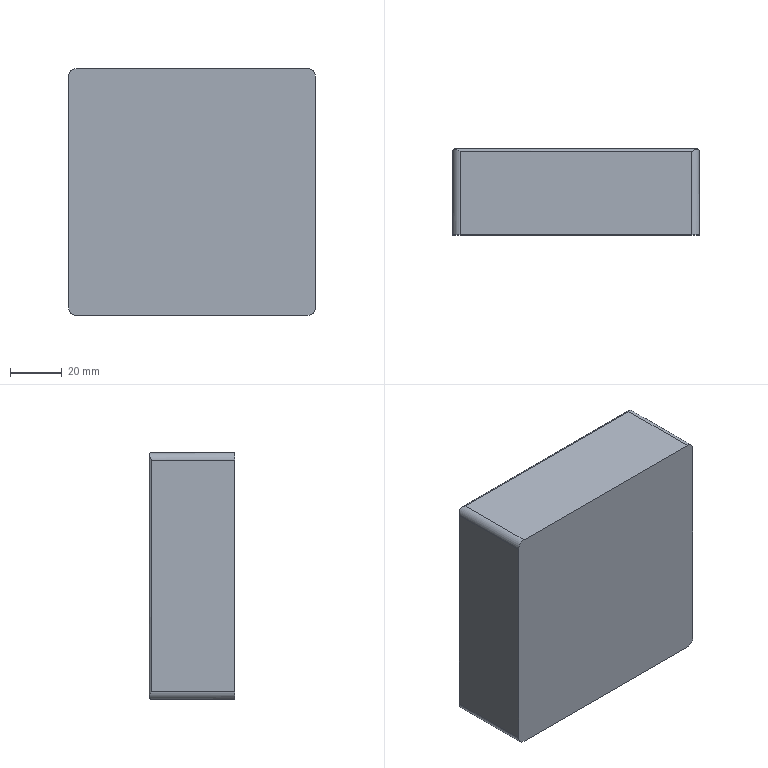Part | SolidWorks | features BaseBody 1 | 1 solid | 20 faces | box 95 x 33 x 95 mm | volume 297490 mm3 | cylinder 9 | plane 6 | cone 5 | commonest cylinder face diameters 2 x5 6 x4
STEP:
#1=CARTESIAN_POINT('',(155.5,-10.5,-46.5));
#2=VERTEX_POINT('',#1);
#3=CARTESIAN_POINT('',(154.5,-10.5,-47.5));
#4=VERTEX_POINT('',#3);
#5=CARTESIAN_POINT('',(154.5,-10.5,-47.5));
#6=DIRECTION('',(-0.7071,0.,-0.7071));
#7=VECTOR('',#6,1000.);
#8=LINE('',#5,#7);
#9=EDGE_CURVE('',#2,#4,#8,.T.);
#10=ORIENTED_EDGE('',*,*,#9,.F.);
#11=CARTESIAN_POINT('',(156.5,-10.5,-47.5));
#12=VERTEX_POINT('',#11);
#13=CARTESIAN_POINT('',(156.5,-10.5,-47.5));
#14=DIRECTION('',(0.7071,0.,-0.7071));
#15=VECTOR('',#14,1000.);
#16=LINE('',#13,#15);
#17=EDGE_CURVE('',#2,#12,#16,.T.);
#18=ORIENTED_EDGE('',*,*,#17,.T.);
#19=CARTESIAN_POINT('',(155.5,-10.5,-47.5));
#20=DIRECTION('',(0.,0.,1.));
#21=DIRECTION('',(-1.,0.,0.));
#22=AXIS2_PLACEMENT_3D('',#19,#20,#21);
#23=CIRCLE('',#22,1.);
#24=EDGE_CURVE('',#4,#12,#23,.T.);
#25=ORIENTED_EDGE('',*,*,#24,.F.);
#26=EDGE_LOOP('',(#10,#18,#25));
#27=FACE_OUTER_BOUND('',#26,.T.);
#28=CARTESIAN_POINT('',(155.5,-10.5,-47.5));
#29=DIRECTION('',(0.,0.,-1.));
#30=DIRECTION('',(-1.,0.,0.));
#31=AXIS2_PLACEMENT_3D('',#28,#29,#30);
#32=CONICAL_SURFACE('',#31,1.,0.7854);
#33=ADVANCED_FACE('',(#27),#32,.F.);
#34=CARTESIAN_POINT('',(182.5,-10.5,-46.5));
#35=VERTEX_POINT('',#34);
#36=CARTESIAN_POINT('',(181.5,-10.5,-47.5));
#37=VERTEX_POINT('',#36);
#38=CARTESIAN_POINT('',(181.5,-10.5,-47.5));
#39=DIRECTION('',(-0.7071,0.,-0.7071));
#40=VECTOR('',#39,1000.);
#41=LINE('',#38,#40);
#42=EDGE_CURVE('',#35,#37,#41,.T.);
#43=ORIENTED_EDGE('',*,*,#42,.F.);
#44=CARTESIAN_POINT('',(183.5,-10.5,-47.5));
#45=VERTEX_POINT('',#44);
#46=CARTESIAN_POINT('',(183.5,-10.5,-47.5));
#47=DIRECTION('',(0.7071,0.,-0.7071));
#48=VECTOR('',#47,1000.);
#49=LINE('',#46,#48);
#50=EDGE_CURVE('',#35,#45,#49,.T.);
#51=ORIENTED_EDGE('',*,*,#50,.T.);
#52=CARTESIAN_POINT('',(182.5,-10.5,-47.5));
#53=DIRECTION('',(0.,0.,1.));
#54=DIRECTION('',(-1.,0.,0.));
#55=AXIS2_PLACEMENT_3D('',#52,#53,#54);
#56=CIRCLE('',#55,1.);
#57=EDGE_CURVE('',#37,#45,#56,.T.);
#58=ORIENTED_EDGE('',*,*,#57,.F.);
#59=EDGE_LOOP('',(#43,#51,#58));
#60=FACE_OUTER_BOUND('',#59,.T.);
#61=CARTESIAN_POINT('',(182.5,-10.5,-47.5));
#62=DIRECTION('',(0.,0.,-1.));
#63=DIRECTION('',(-1.,0.,0.));
#64=AXIS2_PLACEMENT_3D('',#61,#62,#63);
#65=CONICAL_SURFACE('',#64,1.,0.7854);
#66=ADVANCED_FACE('',(#60),#65,.F.);
#67=CARTESIAN_POINT('',(218.,-26.,44.5));
#68=VERTEX_POINT('',#67);
#69=CARTESIAN_POINT('',(215.,-26.,47.5));
#70=VERTEX_POINT('',#69);
#71=CARTESIAN_POINT('',(215.,-26.,44.5));
#72=DIRECTION('',(0.,-1.,0.));
#73=DIRECTION('',(0.,0.,-1.));
#74=AXIS2_PLACEMENT_3D('',#71,#72,#73);
#75=CIRCLE('',#74,3.);
#76=EDGE_CURVE('',#68,#70,#75,.T.);
#77=ORIENTED_EDGE('',*,*,#76,.T.);
#78=CARTESIAN_POINT('',(126.,-26.,47.5));
#79=VERTEX_POINT('',#78);
#80=CARTESIAN_POINT('',(170.5,-26.,47.5));
#81=DIRECTION('',(-1.,0.,0.));
#82=VECTOR('',#81,1000.);
#83=LINE('',#80,#82);
#84=EDGE_CURVE('',#70,#79,#83,.T.);
#85=ORIENTED_EDGE('',*,*,#84,.T.);
#86=CARTESIAN_POINT('',(123.,-26.,44.5));
#87=VERTEX_POINT('',#86);
#88=CARTESIAN_POINT('',(126.,-26.,44.5));
#89=DIRECTION('',(0.,-1.,0.));
#90=DIRECTION('',(0.,0.,-1.));
#91=AXIS2_PLACEMENT_3D('',#88,#89,#90);
#92=CIRCLE('',#91,3.);
#93=EDGE_CURVE('',#79,#87,#92,.T.);
#94=ORIENTED_EDGE('',*,*,#93,.T.);
#95=CARTESIAN_POINT('',(123.,-26.,-44.5));
#96=VERTEX_POINT('',#95);
#97=CARTESIAN_POINT('',(123.,-26.,0.));
#98=DIRECTION('',(0.,0.,-1.));
#99=VECTOR('',#98,1000.);
#100=LINE('',#97,#99);
#101=EDGE_CURVE('',#87,#96,#100,.T.);
#102=ORIENTED_EDGE('',*,*,#101,.T.);
#103=CARTESIAN_POINT('',(126.,-26.,-47.5));
#104=VERTEX_POINT('',#103);
#105=CARTESIAN_POINT('',(126.,-26.,-44.5));
#106=DIRECTION('',(0.,-1.,0.));
#107=DIRECTION('',(0.,0.,-1.));
#108=AXIS2_PLACEMENT_3D('',#105,#106,#107);
#109=CIRCLE('',#108,3.);
#110=EDGE_CURVE('',#96,#104,#109,.T.);
#111=ORIENTED_EDGE('',*,*,#110,.T.);
#112=CARTESIAN_POINT('',(215.,-26.,-47.5));
#113=VERTEX_POINT('',#112);
#114=CARTESIAN_POINT('',(170.5,-26.,-47.5));
#115=DIRECTION('',(1.,0.,0.));
#116=VECTOR('',#115,1000.);
#117=LINE('',#114,#116);
#118=EDGE_CURVE('',#104,#113,#117,.T.);
#119=ORIENTED_EDGE('',*,*,#118,.T.);
#120=CARTESIAN_POINT('',(218.,-26.,-44.5));
#121=VERTEX_POINT('',#120);
#122=CARTESIAN_POINT('',(215.,-26.,-44.5));
#123=DIRECTION('',(0.,-1.,0.));
#124=DIRECTION('',(0.,0.,-1.));
#125=AXIS2_PLACEMENT_3D('',#122,#123,#124);
#126=CIRCLE('',#125,3.);
#127=EDGE_CURVE('',#113,#121,#126,.T.);
#128=ORIENTED_EDGE('',*,*,#127,.T.);
#129=CARTESIAN_POINT('',(218.,-26.,0.));
#130=DIRECTION('',(0.,0.,1.));
#131=VECTOR('',#130,1000.);
#132=LINE('',#129,#131);
#133=EDGE_CURVE('',#121,#68,#132,.T.);
#134=ORIENTED_EDGE('',*,*,#133,.T.);
#135=EDGE_LOOP('',(#77,#85,#94,#102,#111,#119,#128,#134));
#136=FACE_OUTER_BOUND('',#135,.T.);
#137=CARTESIAN_POINT('',(170.5,-26.,0.));
#138=DIRECTION('',(0.,-1.,0.));
#139=DIRECTION('',(0.,0.,-1.));
#140=AXIS2_PLACEMENT_3D('',#137,#138,#139);
#141=PLANE('',#140);
#142=ADVANCED_FACE('',(#136),#141,.T.);
#143=CARTESIAN_POINT('',(215.,6.,47.5));
#144=VERTEX_POINT('',#143);
#145=CARTESIAN_POINT('',(215.,7.,47.5));
#146=DIRECTION('',(0.,1.,0.));
#147=VECTOR('',#146,1000.);
#148=LINE('',#145,#147);
#149=EDGE_CURVE('',#70,#144,#148,.T.);
#150=ORIENTED_EDGE('',*,*,#149,.T.);
#151=CARTESIAN_POINT('',(126.,6.,47.5));
#152=VERTEX_POINT('',#151);
#153=CARTESIAN_POINT('',(126.,6.,47.5));
#154=DIRECTION('',(-1.,0.,0.));
#155=VECTOR('',#154,1000.);
#156=LINE('',#153,#155);
#157=EDGE_CURVE('',#144,#152,#156,.T.);
#158=ORIENTED_EDGE('',*,*,#157,.T.);
#159=CARTESIAN_POINT('',(126.,7.,47.5));
#160=DIRECTION('',(0.,-1.,0.));
#161=VECTOR('',#160,1000.);
#162=LINE('',#159,#161);
#163=EDGE_CURVE('',#152,#79,#162,.T.);
#164=ORIENTED_EDGE('',*,*,#163,.T.);
#165=ORIENTED_EDGE('',*,*,#84,.F.);
#166=EDGE_LOOP('',(#150,#158,#164,#165));
#167=FACE_OUTER_BOUND('',#166,.T.);
#168=CARTESIAN_POINT('',(126.,7.,47.5));
#169=DIRECTION('',(0.,0.,1.));
#170=DIRECTION('',(1.,0.,0.));
#171=AXIS2_PLACEMENT_3D('',#168,#169,#170);
#172=PLANE('',#171);
#173=ADVANCED_FACE('',(#167),#172,.T.);
#174=CARTESIAN_POINT('',(218.,6.,44.5));
#175=VERTEX_POINT('',#174);
#176=CARTESIAN_POINT('',(218.,7.,44.5));
#177=DIRECTION('',(0.,1.,0.));
#178=VECTOR('',#177,1000.);
#179=LINE('',#176,#178);
#180=EDGE_CURVE('',#68,#175,#179,.T.);
#181=ORIENTED_EDGE('',*,*,#180,.T.);
#182=CARTESIAN_POINT('',(217.121,6.993,46.621));
#183=VERTEX_POINT('',#182);
#184=CARTESIAN_POINT('',(218.,6.,44.5));
#185=CARTESIAN_POINT('',(218.,6.053,44.592));
#186=CARTESIAN_POINT('',(217.996,6.108,44.686));
#187=CARTESIAN_POINT('',(217.978,6.214,44.871));
#188=CARTESIAN_POINT('',(217.965,6.266,44.963));
#189=CARTESIAN_POINT('',(217.914,6.421,45.238));
#190=CARTESIAN_POINT('',(217.862,6.52,45.42));
#191=CARTESIAN_POINT('',(217.718,6.705,45.784));
#192=CARTESIAN_POINT('',(217.628,6.789,45.961));
#193=CARTESIAN_POINT('',(217.406,6.923,46.303));
#194=CARTESIAN_POINT('',(217.273,6.974,46.469));
#195=CARTESIAN_POINT('',(217.121,6.993,46.621));
#196=B_SPLINE_CURVE_WITH_KNOTS('',3,(#184,#185,#186,#187,#188,#189,#190,#191,#192,#193,#194,#195),.UNSPECIFIED.,.F.,.F.,(4,2,2,2,2,4),(-0.00001095,0.0003086,0.0006282,0.001267,0.001907,0.002546),.UNSPECIFIED.);
#197=EDGE_CURVE('',#175,#183,#196,.T.);
#198=ORIENTED_EDGE('',*,*,#197,.T.);
#199=CARTESIAN_POINT('',(217.121,6.993,46.621));
#200=CARTESIAN_POINT('',(216.968,6.974,46.774));
#201=CARTESIAN_POINT('',(216.806,6.924,46.904));
#202=CARTESIAN_POINT('',(216.461,6.789,47.128));
#203=CARTESIAN_POINT('',(216.285,6.706,47.218));
#204=CARTESIAN_POINT('',(215.746,6.432,47.431));
#205=CARTESIAN_POINT('',(215.371,6.214,47.5));
#206=CARTESIAN_POINT('',(215.,6.,47.5));
#207=B_SPLINE_CURVE_WITH_KNOTS('',3,(#199,#200,#201,#202,#203,#204,#205,#206),.UNSPECIFIED.,.F.,.F.,(4,2,2,4),(0.,0.0006423,0.001285,0.002569),.UNSPECIFIED.);
#208=EDGE_CURVE('',#183,#144,#207,.T.);
#209=ORIENTED_EDGE('',*,*,#208,.T.);
#210=ORIENTED_EDGE('',*,*,#149,.F.);
#211=ORIENTED_EDGE('',*,*,#76,.F.);
#212=EDGE_LOOP('',(#181,#198,#209,#210,#211));
#213=FACE_OUTER_BOUND('',#212,.T.);
#214=CARTESIAN_POINT('',(215.,7.,44.5));
#215=DIRECTION('',(0.,-1.,0.));
#216=DIRECTION('',(0.,0.,-1.));
#217=AXIS2_PLACEMENT_3D('',#214,#215,#216);
#218=CYLINDRICAL_SURFACE('',#217,3.);
#219=ADVANCED_FACE('',(#213),#218,.T.);
#220=CARTESIAN_POINT('',(218.,6.,-44.5));
#221=VERTEX_POINT('',#220);
#222=CARTESIAN_POINT('',(218.,7.,-44.5));
#223=DIRECTION('',(0.,1.,0.));
#224=VECTOR('',#223,1000.);
#225=LINE('',#222,#224);
#226=EDGE_CURVE('',#121,#221,#225,.T.);
#227=ORIENTED_EDGE('',*,*,#226,.T.);
#228=CARTESIAN_POINT('',(218.,6.,44.5));
#229=DIRECTION('',(0.,0.,1.));
#230=VECTOR('',#229,1000.);
#231=LINE('',#228,#230);
#232=EDGE_CURVE('',#221,#175,#231,.T.);
#233=ORIENTED_EDGE('',*,*,#232,.T.);
#234=ORIENTED_EDGE('',*,*,#180,.F.);
#235=ORIENTED_EDGE('',*,*,#133,.F.);
#236=EDGE_LOOP('',(#227,#233,#234,#235));
#237=FACE_OUTER_BOUND('',#236,.T.);
#238=CARTESIAN_POINT('',(218.,7.,44.5));
#239=DIRECTION('',(1.,0.,0.));
#240=DIRECTION('',(0.,0.,-1.));
#241=AXIS2_PLACEMENT_3D('',#238,#239,#240);
#242=PLANE('',#241);
#243=ADVANCED_FACE('',(#237),#242,.T.);
#244=ORIENTED_EDGE('',*,*,#127,.F.);
#245=CARTESIAN_POINT('',(215.,6.,-47.5));
#246=VERTEX_POINT('',#245);
#247=CARTESIAN_POINT('',(215.,7.,-47.5));
#248=DIRECTION('',(0.,1.,0.));
#249=VECTOR('',#248,1000.);
#250=LINE('',#247,#249);
#251=EDGE_CURVE('',#113,#246,#250,.T.);
#252=ORIENTED_EDGE('',*,*,#251,.T.);
#253=CARTESIAN_POINT('',(217.121,6.993,-46.621));
#254=VERTEX_POINT('',#253);
#255=CARTESIAN_POINT('',(215.,6.,-47.5));
#256=CARTESIAN_POINT('',(215.092,6.053,-47.5));
#257=CARTESIAN_POINT('',(215.186,6.108,-47.496));
#258=CARTESIAN_POINT('',(215.371,6.214,-47.478));
#259=CARTESIAN_POINT('',(215.463,6.266,-47.465));
#260=CARTESIAN_POINT('',(215.738,6.421,-47.414));
#261=CARTESIAN_POINT('',(215.92,6.52,-47.362));
#262=CARTESIAN_POINT('',(216.284,6.705,-47.218));
#263=CARTESIAN_POINT('',(216.461,6.789,-47.128));
#264=CARTESIAN_POINT('',(216.803,6.923,-46.906));
#265=CARTESIAN_POINT('',(216.969,6.974,-46.773));
#266=CARTESIAN_POINT('',(217.121,6.993,-46.621));
#267=B_SPLINE_CURVE_WITH_KNOTS('',3,(#255,#256,#257,#258,#259,#260,#261,#262,#263,#264,#265,#266),.UNSPECIFIED.,.F.,.F.,(4,2,2,2,2,4),(-0.00001095,0.0003086,0.0006282,0.001267,0.001907,0.002546),.UNSPECIFIED.);
#268=EDGE_CURVE('',#246,#254,#267,.T.);
#269=ORIENTED_EDGE('',*,*,#268,.T.);
#270=CARTESIAN_POINT('',(217.121,6.993,-46.621));
#271=CARTESIAN_POINT('',(217.274,6.974,-46.468));
#272=CARTESIAN_POINT('',(217.404,6.924,-46.306));
#273=CARTESIAN_POINT('',(217.628,6.789,-45.961));
#274=CARTESIAN_POINT('',(217.718,6.706,-45.785));
#275=CARTESIAN_POINT('',(217.931,6.432,-45.246));
#276=CARTESIAN_POINT('',(218.,6.214,-44.871));
#277=CARTESIAN_POINT('',(218.,6.,-44.5));
#278=B_SPLINE_CURVE_WITH_KNOTS('',3,(#270,#271,#272,#273,#274,#275,#276,#277),.UNSPECIFIED.,.F.,.F.,(4,2,2,4),(0.,0.0006423,0.001285,0.002569),.UNSPECIFIED.);
#279=EDGE_CURVE('',#254,#221,#278,.T.);
#280=ORIENTED_EDGE('',*,*,#279,.T.);
#281=ORIENTED_EDGE('',*,*,#226,.F.);
#282=EDGE_LOOP('',(#244,#252,#269,#280,#281));
#283=FACE_OUTER_BOUND('',#282,.T.);
#284=CARTESIAN_POINT('',(215.,7.,-44.5));
#285=DIRECTION('',(0.,-1.,0.));
#286=DIRECTION('',(0.,0.,-1.));
#287=AXIS2_PLACEMENT_3D('',#284,#285,#286);
#288=CYLINDRICAL_SURFACE('',#287,3.);
#289=ADVANCED_FACE('',(#283),#288,.T.);
#290=CARTESIAN_POINT('',(126.,6.,-47.5));
#291=VERTEX_POINT('',#290);
#292=CARTESIAN_POINT('',(182.5,6.,-47.5));
#293=VERTEX_POINT('',#292);
#294=CARTESIAN_POINT('',(215.,6.,-47.5));
#295=DIRECTION('',(1.,0.,0.));
#296=VECTOR('',#295,1000.);
#297=LINE('',#294,#296);
#298=EDGE_CURVE('',#291,#293,#297,.T.);
#299=ORIENTED_EDGE('',*,*,#298,.T.);
#300=CARTESIAN_POINT('',(215.,6.,-47.5));
#301=DIRECTION('',(1.,0.,0.));
#302=VECTOR('',#301,1000.);
#303=LINE('',#300,#302);
#304=EDGE_CURVE('',#293,#246,#303,.T.);
#305=ORIENTED_EDGE('',*,*,#304,.T.);
#306=ORIENTED_EDGE('',*,*,#251,.F.);
#307=ORIENTED_EDGE('',*,*,#118,.F.);
#308=CARTESIAN_POINT('',(126.,7.,-47.5));
#309=DIRECTION('',(0.,1.,0.));
#310=VECTOR('',#309,1000.);
#311=LINE('',#308,#310);
#312=EDGE_CURVE('',#104,#291,#311,.T.);
#313=ORIENTED_EDGE('',*,*,#312,.T.);
#314=EDGE_LOOP('',(#299,#305,#306,#307,#313));
#315=FACE_OUTER_BOUND('',#314,.T.);
#316=ORIENTED_EDGE('',*,*,#24,.T.);
#317=CARTESIAN_POINT('',(155.5,-10.5,-47.5));
#318=DIRECTION('',(0.,0.,1.));
#319=DIRECTION('',(-1.,0.,0.));
#320=AXIS2_PLACEMENT_3D('',#317,#318,#319);
#321=CIRCLE('',#320,1.);
#322=EDGE_CURVE('',#12,#4,#321,.T.);
#323=ORIENTED_EDGE('',*,*,#322,.T.);
#324=EDGE_LOOP('',(#316,#323));
#325=FACE_BOUND('',#324,.T.);
#326=ORIENTED_EDGE('',*,*,#57,.T.);
#327=CARTESIAN_POINT('',(182.5,-10.5,-47.5));
#328=DIRECTION('',(0.,0.,1.));
#329=DIRECTION('',(-1.,0.,0.));
#330=AXIS2_PLACEMENT_3D('',#327,#328,#329);
#331=CIRCLE('',#330,1.);
#332=EDGE_CURVE('',#45,#37,#331,.T.);
#333=ORIENTED_EDGE('',*,*,#332,.T.);
#334=EDGE_LOOP('',(#326,#333));
#335=FACE_BOUND('',#334,.T.);
#336=CARTESIAN_POINT('',(215.,7.,-47.5));
#337=DIRECTION('',(0.,0.,-1.));
#338=DIRECTION('',(-1.,0.,0.));
#339=AXIS2_PLACEMENT_3D('',#336,#337,#338);
#340=PLANE('',#339);
#341=ADVANCED_FACE('',(#315,#325,#335),#340,.T.);
#342=CARTESIAN_POINT('',(123.,6.,-44.5));
#343=VERTEX_POINT('',#342);
#344=CARTESIAN_POINT('',(123.,7.,-44.5));
#345=DIRECTION('',(0.,1.,0.));
#346=VECTOR('',#345,1000.);
#347=LINE('',#344,#346);
#348=EDGE_CURVE('',#96,#343,#347,.T.);
#349=ORIENTED_EDGE('',*,*,#348,.T.);
#350=CARTESIAN_POINT('',(123.879,6.993,-46.621));
#351=VERTEX_POINT('',#350);
#352=CARTESIAN_POINT('',(123.,6.,-44.5));
#353=CARTESIAN_POINT('',(123.,6.214,-44.871));
#354=CARTESIAN_POINT('',(123.069,6.432,-45.247));
#355=CARTESIAN_POINT('',(123.282,6.706,-45.785));
#356=CARTESIAN_POINT('',(123.372,6.789,-45.961));
#357=CARTESIAN_POINT('',(123.596,6.924,-46.306));
#358=CARTESIAN_POINT('',(123.726,6.974,-46.468));
#359=CARTESIAN_POINT('',(123.879,6.993,-46.621));
#360=B_SPLINE_CURVE_WITH_KNOTS('',3,(#352,#353,#354,#355,#356,#357,#358,#359),.UNSPECIFIED.,.F.,.F.,(4,2,2,4),(-0.00001095,0.001275,0.001919,0.002562),.UNSPECIFIED.);
#361=EDGE_CURVE('',#343,#351,#360,.T.);
#362=ORIENTED_EDGE('',*,*,#361,.T.);
#363=CARTESIAN_POINT('',(123.879,6.993,-46.621));
#364=CARTESIAN_POINT('',(124.032,6.974,-46.774));
#365=CARTESIAN_POINT('',(124.194,6.924,-46.904));
#366=CARTESIAN_POINT('',(124.539,6.789,-47.128));
#367=CARTESIAN_POINT('',(124.715,6.706,-47.218));
#368=CARTESIAN_POINT('',(125.254,6.432,-47.431));
#369=CARTESIAN_POINT('',(125.629,6.214,-47.5));
#370=CARTESIAN_POINT('',(126.,6.,-47.5));
#371=B_SPLINE_CURVE_WITH_KNOTS('',3,(#363,#364,#365,#366,#367,#368,#369,#370),.UNSPECIFIED.,.F.,.F.,(4,2,2,4),(0.,0.0006423,0.001285,0.002569),.UNSPECIFIED.);
#372=EDGE_CURVE('',#351,#291,#371,.T.);
#373=ORIENTED_EDGE('',*,*,#372,.T.);
#374=ORIENTED_EDGE('',*,*,#312,.F.);
#375=ORIENTED_EDGE('',*,*,#110,.F.);
#376=EDGE_LOOP('',(#349,#362,#373,#374,#375));
#377=FACE_OUTER_BOUND('',#376,.T.);
#378=CARTESIAN_POINT('',(126.,7.,-44.5));
#379=DIRECTION('',(0.,-1.,0.));
#380=DIRECTION('',(0.,0.,-1.));
#381=AXIS2_PLACEMENT_3D('',#378,#379,#380);
#382=CYLINDRICAL_SURFACE('',#381,3.);
#383=ADVANCED_FACE('',(#377),#382,.T.);
#384=CARTESIAN_POINT('',(123.,6.,44.5));
#385=VERTEX_POINT('',#384);
#386=CARTESIAN_POINT('',(123.,7.,44.5));
#387=DIRECTION('',(0.,1.,0.));
#388=VECTOR('',#387,1000.);
#389=LINE('',#386,#388);
#390=EDGE_CURVE('',#87,#385,#389,.T.);
#391=ORIENTED_EDGE('',*,*,#390,.T.);
#392=CARTESIAN_POINT('',(123.,6.,0.));
#393=DIRECTION('',(0.,0.,-1.));
#394=VECTOR('',#393,1000.);
#395=LINE('',#392,#394);
#396=EDGE_CURVE('',#385,#343,#395,.T.);
#397=ORIENTED_EDGE('',*,*,#396,.T.);
#398=ORIENTED_EDGE('',*,*,#348,.F.);
#399=ORIENTED_EDGE('',*,*,#101,.F.);
#400=EDGE_LOOP('',(#391,#397,#398,#399));
#401=FACE_OUTER_BOUND('',#400,.T.);
#402=CARTESIAN_POINT('',(123.,7.,0.));
#403=DIRECTION('',(-1.,0.,0.));
#404=DIRECTION('',(0.,0.,1.));
#405=AXIS2_PLACEMENT_3D('',#402,#403,#404);
#406=PLANE('',#405);
#407=ADVANCED_FACE('',(#401),#406,.T.);
#408=ORIENTED_EDGE('',*,*,#93,.F.);
#409=ORIENTED_EDGE('',*,*,#163,.F.);
#410=CARTESIAN_POINT('',(123.879,6.993,46.621));
#411=VERTEX_POINT('',#410);
#412=CARTESIAN_POINT('',(126.,6.,47.5));
#413=CARTESIAN_POINT('',(125.629,6.214,47.5));
#414=CARTESIAN_POINT('',(125.253,6.432,47.431));
#415=CARTESIAN_POINT('',(124.715,6.706,47.218));
#416=CARTESIAN_POINT('',(124.539,6.789,47.128));
#417=CARTESIAN_POINT('',(124.194,6.924,46.904));
#418=CARTESIAN_POINT('',(124.032,6.974,46.774));
#419=CARTESIAN_POINT('',(123.879,6.993,46.621));
#420=B_SPLINE_CURVE_WITH_KNOTS('',3,(#412,#413,#414,#415,#416,#417,#418,#419),.UNSPECIFIED.,.F.,.F.,(4,2,2,4),(-0.00001095,0.001275,0.001919,0.002562),.UNSPECIFIED.);
#421=EDGE_CURVE('',#152,#411,#420,.T.);
#422=ORIENTED_EDGE('',*,*,#421,.T.);
#423=CARTESIAN_POINT('',(123.879,6.993,46.621));
#424=CARTESIAN_POINT('',(123.726,6.974,46.468));
#425=CARTESIAN_POINT('',(123.596,6.924,46.306));
#426=CARTESIAN_POINT('',(123.372,6.789,45.961));
#427=CARTESIAN_POINT('',(123.282,6.706,45.785));
#428=CARTESIAN_POINT('',(123.069,6.432,45.246));
#429=CARTESIAN_POINT('',(123.,6.214,44.871));
#430=CARTESIAN_POINT('',(123.,6.,44.5));
#431=B_SPLINE_CURVE_WITH_KNOTS('',3,(#423,#424,#425,#426,#427,#428,#429,#430),.UNSPECIFIED.,.F.,.F.,(4,2,2,4),(0.,0.0006423,0.001285,0.002569),.UNSPECIFIED.);
#432=EDGE_CURVE('',#411,#385,#431,.T.);
#433=ORIENTED_EDGE('',*,*,#432,.T.);
#434=ORIENTED_EDGE('',*,*,#390,.F.);
#435=EDGE_LOOP('',(#408,#409,#422,#433,#434));
#436=FACE_OUTER_BOUND('',#435,.T.);
#437=CARTESIAN_POINT('',(126.,7.,44.5));
#438=DIRECTION('',(0.,-1.,0.));
#439=DIRECTION('',(0.,0.,-1.));
#440=AXIS2_PLACEMENT_3D('',#437,#438,#439);
#441=CYLINDRICAL_SURFACE('',#440,3.);
#442=ADVANCED_FACE('',(#436),#441,.T.);
#443=ORIENTED_EDGE('',*,*,#421,.F.);
#444=ORIENTED_EDGE('',*,*,#157,.F.);
#445=ORIENTED_EDGE('',*,*,#208,.F.);
#446=CARTESIAN_POINT('',(217.,7.,46.5));
#447=VERTEX_POINT('',#446);
#448=CARTESIAN_POINT('',(217.121,6.993,46.621));
#449=CARTESIAN_POINT('',(217.081,6.998,46.581));
#450=CARTESIAN_POINT('',(217.041,7.,46.541));
#451=CARTESIAN_POINT('',(217.,7.,46.5));
#452=(BOUNDED_CURVE()B_SPLINE_CURVE(3,(#448,#449,#450,#451),.UNSPECIFIED.,.F.,.F.)B_SPLINE_CURVE_WITH_KNOTS((4,4),(4.591,4.712),.UNSPECIFIED.)CURVE()GEOMETRIC_REPRESENTATION_ITEM()RATIONAL_B_SPLINE_CURVE((1.,0.9988,0.9988,1.))REPRESENTATION_ITEM(''));
#453=EDGE_CURVE('',#183,#447,#452,.T.);
#454=ORIENTED_EDGE('',*,*,#453,.T.);
#455=CARTESIAN_POINT('',(124.,7.,46.5));
#456=VERTEX_POINT('',#455);
#457=CARTESIAN_POINT('',(218.,7.,46.5));
#458=DIRECTION('',(-1.,0.,0.));
#459=VECTOR('',#458,1000.);
#460=LINE('',#457,#459);
#461=EDGE_CURVE('',#447,#456,#460,.T.);
#462=ORIENTED_EDGE('',*,*,#461,.T.);
#463=CARTESIAN_POINT('',(124.,7.,46.5));
#464=CARTESIAN_POINT('',(123.959,7.,46.541));
#465=CARTESIAN_POINT('',(123.919,6.998,46.581));
#466=CARTESIAN_POINT('',(123.879,6.993,46.621));
#467=(BOUNDED_CURVE()B_SPLINE_CURVE(3,(#463,#464,#465,#466),.UNSPECIFIED.,.F.,.T.)B_SPLINE_CURVE_WITH_KNOTS((4,4),(4.712,4.834),.UNSPECIFIED.)CURVE()GEOMETRIC_REPRESENTATION_ITEM()RATIONAL_B_SPLINE_CURVE((1.,0.9988,0.9988,1.))REPRESENTATION_ITEM(''));
#468=EDGE_CURVE('',#456,#411,#467,.T.);
#469=ORIENTED_EDGE('',*,*,#468,.T.);
#470=EDGE_LOOP('',(#443,#444,#445,#454,#462,#469));
#471=FACE_OUTER_BOUND('',#470,.T.);
#472=CARTESIAN_POINT('',(218.,6.,46.5));
#473=DIRECTION('',(-1.,0.,0.));
#474=DIRECTION('',(0.,0.,1.));
#475=AXIS2_PLACEMENT_3D('',#472,#473,#474);
#476=CYLINDRICAL_SURFACE('',#475,1.);
#477=ADVANCED_FACE('',(#471),#476,.T.);
#478=ORIENTED_EDGE('',*,*,#232,.F.);
#479=ORIENTED_EDGE('',*,*,#279,.F.);
#480=CARTESIAN_POINT('',(217.,7.,-46.5));
#481=VERTEX_POINT('',#480);
#482=CARTESIAN_POINT('',(217.121,6.993,-46.621));
#483=CARTESIAN_POINT('',(217.081,6.998,-46.581));
#484=CARTESIAN_POINT('',(217.041,7.,-46.541));
#485=CARTESIAN_POINT('',(217.,7.,-46.5));
#486=(BOUNDED_CURVE()B_SPLINE_CURVE(3,(#482,#483,#484,#485),.UNSPECIFIED.,.F.,.F.)B_SPLINE_CURVE_WITH_KNOTS((4,4),(1.449,1.571),.UNSPECIFIED.)CURVE()GEOMETRIC_REPRESENTATION_ITEM()RATIONAL_B_SPLINE_CURVE((1.,0.9988,0.9988,1.))REPRESENTATION_ITEM(''));
#487=EDGE_CURVE('',#254,#481,#486,.T.);
#488=ORIENTED_EDGE('',*,*,#487,.T.);
#489=CARTESIAN_POINT('',(217.,7.,47.5));
#490=DIRECTION('',(0.,0.,1.));
#491=VECTOR('',#490,1000.);
#492=LINE('',#489,#491);
#493=EDGE_CURVE('',#481,#447,#492,.T.);
#494=ORIENTED_EDGE('',*,*,#493,.T.);
#495=ORIENTED_EDGE('',*,*,#453,.F.);
#496=ORIENTED_EDGE('',*,*,#197,.F.);
#497=EDGE_LOOP('',(#478,#479,#488,#494,#495,#496));
#498=FACE_OUTER_BOUND('',#497,.T.);
#499=CARTESIAN_POINT('',(217.,6.,47.5));
#500=DIRECTION('',(0.,0.,-1.));
#501=DIRECTION('',(-1.,0.,0.));
#502=AXIS2_PLACEMENT_3D('',#499,#500,#501);
#503=CYLINDRICAL_SURFACE('',#502,1.);
#504=ADVANCED_FACE('',(#498),#503,.T.);
#505=ORIENTED_EDGE('',*,*,#268,.F.);
#506=ORIENTED_EDGE('',*,*,#304,.F.);
#507=CARTESIAN_POINT('',(182.5,7.,-46.5));
#508=VERTEX_POINT('',#507);
#509=CARTESIAN_POINT('',(182.5,6.,-47.5));
#510=CARTESIAN_POINT('',(182.594,6.,-47.5));
#511=CARTESIAN_POINT('',(182.69,6.013,-47.5));
#512=CARTESIAN_POINT('',(182.87,6.068,-47.498));
#513=CARTESIAN_POINT('',(182.957,6.11,-47.496));
#514=CARTESIAN_POINT('',(183.104,6.228,-47.475));
#515=CARTESIAN_POINT('',(183.163,6.307,-47.456));
#516=CARTESIAN_POINT('',(183.217,6.475,-47.385));
#517=CARTESIAN_POINT('',(183.209,6.561,-47.333));
#518=CARTESIAN_POINT('',(183.156,6.7,-47.219));
#519=CARTESIAN_POINT('',(183.111,6.759,-47.156));
#520=CARTESIAN_POINT('',(183.008,6.853,-47.028));
#521=CARTESIAN_POINT('',(182.95,6.889,-46.963));
#522=CARTESIAN_POINT('',(182.768,6.974,-46.768));
#523=CARTESIAN_POINT('',(182.633,7.,-46.633));
#524=CARTESIAN_POINT('',(182.5,7.,-46.5));
#525=B_SPLINE_CURVE_WITH_KNOTS('',3,(#509,#510,#511,#512,#513,#514,#515,#516,#517,#518,#519,#520,#521,#522,#523,#524),.UNSPECIFIED.,.F.,.F.,(4,2,2,2,2,2,2,4),(0.0004405,0.000723,0.001006,0.001288,0.001571,0.001853,0.002136,0.002701),.UNSPECIFIED.);
#526=EDGE_CURVE('',#293,#508,#525,.T.);
#527=ORIENTED_EDGE('',*,*,#526,.T.);
#528=CARTESIAN_POINT('',(218.,7.,-46.5));
#529=DIRECTION('',(1.,0.,0.));
#530=VECTOR('',#529,1000.);
#531=LINE('',#528,#530);
#532=EDGE_CURVE('',#508,#481,#531,.T.);
#533=ORIENTED_EDGE('',*,*,#532,.T.);
#534=ORIENTED_EDGE('',*,*,#487,.F.);
#535=EDGE_LOOP('',(#505,#506,#527,#533,#534));
#536=FACE_OUTER_BOUND('',#535,.T.);
#537=CARTESIAN_POINT('',(218.,6.,-46.5));
#538=DIRECTION('',(-1.,0.,0.));
#539=DIRECTION('',(0.,0.,1.));
#540=AXIS2_PLACEMENT_3D('',#537,#538,#539);
#541=CYLINDRICAL_SURFACE('',#540,1.);
#542=ADVANCED_FACE('',(#536),#541,.T.);
#543=CARTESIAN_POINT('',(124.,7.,-46.5));
#544=VERTEX_POINT('',#543);
#545=CARTESIAN_POINT('',(123.879,6.993,-46.621));
#546=CARTESIAN_POINT('',(123.919,6.998,-46.581));
#547=CARTESIAN_POINT('',(123.959,7.,-46.541));
#548=CARTESIAN_POINT('',(124.,7.,-46.5));
#549=(BOUNDED_CURVE()B_SPLINE_CURVE(3,(#545,#546,#547,#548),.UNSPECIFIED.,.F.,.T.)B_SPLINE_CURVE_WITH_KNOTS((4,4),(1.449,1.571),.UNSPECIFIED.)CURVE()GEOMETRIC_REPRESENTATION_ITEM()RATIONAL_B_SPLINE_CURVE((1.,0.9988,0.9988,1.))REPRESENTATION_ITEM(''));
#550=EDGE_CURVE('',#351,#544,#549,.T.);
#551=ORIENTED_EDGE('',*,*,#550,.T.);
#552=CARTESIAN_POINT('',(218.,7.,-46.5));
#553=DIRECTION('',(1.,0.,0.));
#554=VECTOR('',#553,1000.);
#555=LINE('',#552,#554);
#556=EDGE_CURVE('',#544,#508,#555,.T.);
#557=ORIENTED_EDGE('',*,*,#556,.T.);
#558=CARTESIAN_POINT('',(182.5,7.,-46.5));
#559=CARTESIAN_POINT('',(182.366,7.,-46.634));
#560=CARTESIAN_POINT('',(182.232,6.974,-46.768));
#561=CARTESIAN_POINT('',(182.05,6.889,-46.963));
#562=CARTESIAN_POINT('',(181.992,6.853,-47.028));
#563=CARTESIAN_POINT('',(181.889,6.759,-47.156));
#564=CARTESIAN_POINT('',(181.844,6.7,-47.219));
#565=CARTESIAN_POINT('',(181.791,6.561,-47.333));
#566=CARTESIAN_POINT('',(181.783,6.475,-47.385));
#567=CARTESIAN_POINT('',(181.837,6.307,-47.456));
#568=CARTESIAN_POINT('',(181.896,6.228,-47.475));
#569=CARTESIAN_POINT('',(182.043,6.11,-47.496));
#570=CARTESIAN_POINT('',(182.13,6.068,-47.498));
#571=CARTESIAN_POINT('',(182.31,6.013,-47.5));
#572=CARTESIAN_POINT('',(182.406,6.,-47.5));
#573=CARTESIAN_POINT('',(182.5,6.,-47.5));
#574=B_SPLINE_CURVE_WITH_KNOTS('',3,(#558,#559,#560,#561,#562,#563,#564,#565,#566,#567,#568,#569,#570,#571,#572,#573),.UNSPECIFIED.,.F.,.F.,(4,2,2,2,2,2,2,4),(-0.000000019,0.0005676,0.0008514,0.001135,0.001419,0.001703,0.001987,0.00227),.UNSPECIFIED.);
#575=EDGE_CURVE('',#508,#293,#574,.T.);
#576=ORIENTED_EDGE('',*,*,#575,.T.);
#577=ORIENTED_EDGE('',*,*,#298,.F.);
#578=ORIENTED_EDGE('',*,*,#372,.F.);
#579=EDGE_LOOP('',(#551,#557,#576,#577,#578));
#580=FACE_OUTER_BOUND('',#579,.T.);
#581=CARTESIAN_POINT('',(218.,6.,-46.5));
#582=DIRECTION('',(-1.,0.,0.));
#583=DIRECTION('',(0.,0.,1.));
#584=AXIS2_PLACEMENT_3D('',#581,#582,#583);
#585=CYLINDRICAL_SURFACE('',#584,1.);
#586=ADVANCED_FACE('',(#580),#585,.T.);
#587=ORIENTED_EDGE('',*,*,#17,.F.);
#588=ORIENTED_EDGE('',*,*,#9,.T.);
#589=ORIENTED_EDGE('',*,*,#322,.F.);
#590=EDGE_LOOP('',(#587,#588,#589));
#591=FACE_OUTER_BOUND('',#590,.T.);
#592=CARTESIAN_POINT('',(155.5,-10.5,-47.5));
#593=DIRECTION('',(0.,0.,-1.));
#594=DIRECTION('',(-1.,0.,0.));
#595=AXIS2_PLACEMENT_3D('',#592,#593,#594);
#596=CONICAL_SURFACE('',#595,1.,0.7854);
#597=ADVANCED_FACE('',(#591),#596,.F.);
#598=ORIENTED_EDGE('',*,*,#50,.F.);
#599=ORIENTED_EDGE('',*,*,#42,.T.);
#600=ORIENTED_EDGE('',*,*,#332,.F.);
#601=EDGE_LOOP('',(#598,#599,#600));
#602=FACE_OUTER_BOUND('',#601,.T.);
#603=CARTESIAN_POINT('',(182.5,-10.5,-47.5));
#604=DIRECTION('',(0.,0.,-1.));
#605=DIRECTION('',(-1.,0.,0.));
#606=AXIS2_PLACEMENT_3D('',#603,#604,#605);
#607=CONICAL_SURFACE('',#606,1.,0.7854);
#608=ADVANCED_FACE('',(#602),#607,.F.);
#609=ORIENTED_EDGE('',*,*,#468,.F.);
#610=CARTESIAN_POINT('',(124.,7.,47.5));
#611=DIRECTION('',(0.,0.,-1.));
#612=VECTOR('',#611,1000.);
#613=LINE('',#610,#612);
#614=EDGE_CURVE('',#456,#544,#613,.T.);
#615=ORIENTED_EDGE('',*,*,#614,.T.);
#616=ORIENTED_EDGE('',*,*,#550,.F.);
#617=ORIENTED_EDGE('',*,*,#361,.F.);
#618=ORIENTED_EDGE('',*,*,#396,.F.);
#619=ORIENTED_EDGE('',*,*,#432,.F.);
#620=EDGE_LOOP('',(#609,#615,#616,#617,#618,#619));
#621=FACE_OUTER_BOUND('',#620,.T.);
#622=CARTESIAN_POINT('',(124.,6.,47.5));
#623=DIRECTION('',(0.,0.,-1.));
#624=DIRECTION('',(-1.,0.,0.));
#625=AXIS2_PLACEMENT_3D('',#622,#623,#624);
#626=CYLINDRICAL_SURFACE('',#625,1.);
#627=ADVANCED_FACE('',(#621),#626,.T.);
#628=ORIENTED_EDGE('',*,*,#614,.F.);
#629=ORIENTED_EDGE('',*,*,#461,.F.);
#630=ORIENTED_EDGE('',*,*,#493,.F.);
#631=ORIENTED_EDGE('',*,*,#532,.F.);
#632=ORIENTED_EDGE('',*,*,#556,.F.);
#633=EDGE_LOOP('',(#628,#629,#630,#631,#632));
#634=FACE_OUTER_BOUND('',#633,.T.);
#635=CARTESIAN_POINT('',(170.5,7.,0.));
#636=DIRECTION('',(0.,-1.,0.));
#637=DIRECTION('',(0.,0.,-1.));
#638=AXIS2_PLACEMENT_3D('',#635,#636,#637);
#639=PLANE('',#638);
#640=ADVANCED_FACE('',(#634),#639,.F.);
#641=ORIENTED_EDGE('',*,*,#526,.F.);
#642=ORIENTED_EDGE('',*,*,#575,.F.);
#643=EDGE_LOOP('',(#641,#642));
#644=FACE_OUTER_BOUND('',#643,.T.);
#645=CARTESIAN_POINT('',(182.5,7.,-47.506));
#646=DIRECTION('',(0.,0.,-1.));
#647=DIRECTION('',(0.,1.,0.));
#648=AXIS2_PLACEMENT_3D('',#645,#646,#647);
#649=CONICAL_SURFACE('',#648,1.006,0.7854);
#650=ADVANCED_FACE('',(#644),#649,.F.);
#651=CLOSED_SHELL('',(#33,#66,#142,#173,#219,#243,#289,#341,#383,#407,#442,#477,#504,#542,#586,#597,#608,#627,#640,#650));
#652=MANIFOLD_SOLID_BREP('',#651);
#653=CARTESIAN_POINT('',(0.,0.,0.));
#654=DIRECTION('',(0.,0.,1.));
#655=DIRECTION('',(1.,0.,0.));
#656=AXIS2_PLACEMENT_3D('',#653,#654,#655);
#657=(LENGTH_UNIT()NAMED_UNIT(*)SI_UNIT(.MILLI.,.METRE.));
#658=UNCERTAINTY_MEASURE_WITH_UNIT(LENGTH_MEASURE(0.00001),#657,'','');
#659=(NAMED_UNIT(*)PLANE_ANGLE_UNIT()SI_UNIT($,.RADIAN.));
#660=(NAMED_UNIT(*)SI_UNIT($,.STERADIAN.)SOLID_ANGLE_UNIT());
#661=(GEOMETRIC_REPRESENTATION_CONTEXT(3)GLOBAL_UNCERTAINTY_ASSIGNED_CONTEXT((#658))GLOBAL_UNIT_ASSIGNED_CONTEXT((#657,#659,#660))REPRESENTATION_CONTEXT('',''));
#662=ADVANCED_BREP_SHAPE_REPRESENTATION('',(#652,#656),#661);